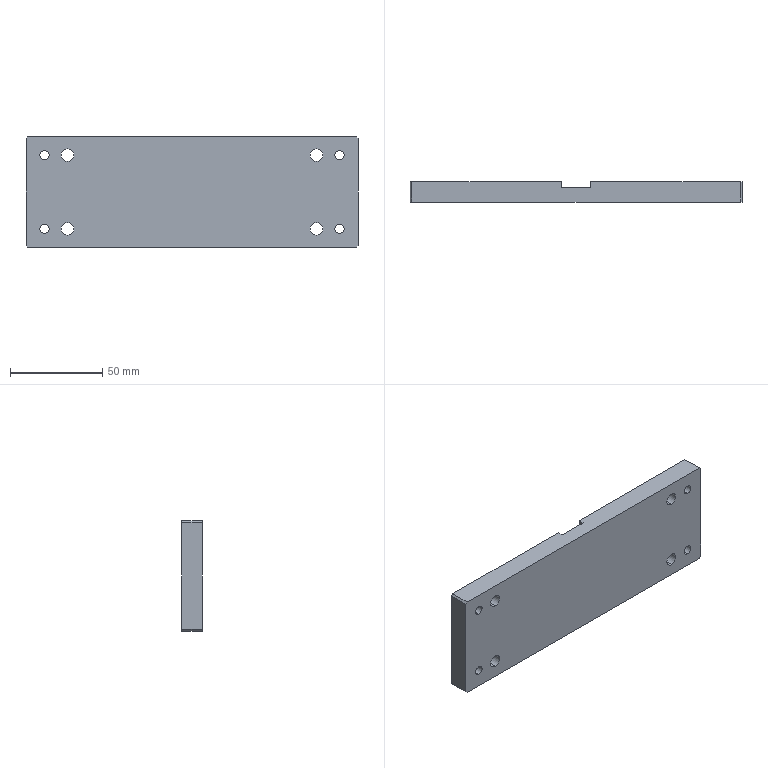Part | STEP file | PN_0011 Plate 1_Default | 1 solid | 30 faces | box 180 x 11 x 60 mm | volume 113436 mm3 | cylinder 16 | plane 14 | commonest cylinder face diameters 5 x8 6.8 x8